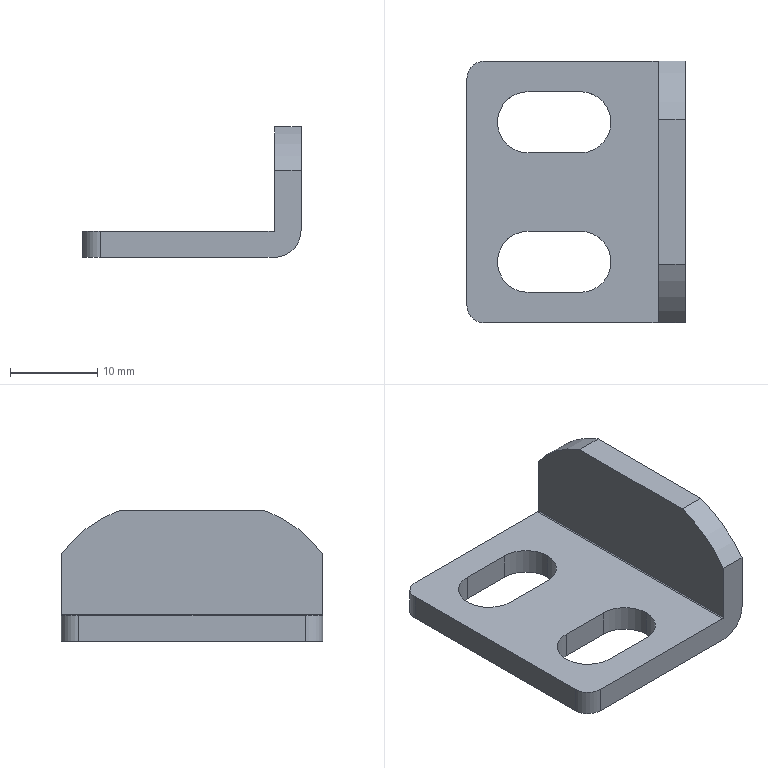Part | STEP file | X Limit Switch Bracket | 1 solid | 24 faces | box 25 x 30 x 15 mm | volume 2701 mm3 | cylinder 12 | plane 12 | commonest cylinder face diameters 7 x6 4 x2 28.772 x2 0.2 x1 6.2 x1
STEP:
#1=CARTESIAN_POINT('',(-2.594,-41.207,-3.));
#2=VERTEX_POINT('',#1);
#3=CARTESIAN_POINT('',(-6.094,-37.707,-3.));
#4=VERTEX_POINT('',#3);
#5=CARTESIAN_POINT('',(-6.094,-41.207,-3.));
#6=DIRECTION('',(0.,0.,1.));
#7=DIRECTION('',(1.,0.,0.));
#8=AXIS2_PLACEMENT_3D('',#5,#6,#7);
#9=CIRCLE('',#8,3.5);
#10=EDGE_CURVE('',#2,#4,#9,.T.);
#11=ORIENTED_EDGE('',*,*,#10,.F.);
#12=CARTESIAN_POINT('',(-2.594,-41.207,0.));
#13=VERTEX_POINT('',#12);
#14=CARTESIAN_POINT('',(-2.594,-41.207,-10.));
#15=DIRECTION('',(0.,0.,1.));
#16=VECTOR('',#15,1000.);
#17=LINE('',#14,#16);
#18=EDGE_CURVE('',#2,#13,#17,.T.);
#19=ORIENTED_EDGE('',*,*,#18,.T.);
#20=CARTESIAN_POINT('',(-6.094,-37.707,0.));
#21=VERTEX_POINT('',#20);
#22=CARTESIAN_POINT('',(-6.094,-41.207,0.));
#23=DIRECTION('',(0.,0.,-1.));
#24=DIRECTION('',(1.,0.,0.));
#25=AXIS2_PLACEMENT_3D('',#22,#23,#24);
#26=CIRCLE('',#25,3.5);
#27=EDGE_CURVE('',#21,#13,#26,.T.);
#28=ORIENTED_EDGE('',*,*,#27,.F.);
#29=CARTESIAN_POINT('',(-6.094,-37.707,-10.));
#30=DIRECTION('',(0.,0.,1.));
#31=VECTOR('',#30,1000.);
#32=LINE('',#29,#31);
#33=EDGE_CURVE('',#4,#21,#32,.T.);
#34=ORIENTED_EDGE('',*,*,#33,.F.);
#35=EDGE_LOOP('',(#11,#19,#28,#34));
#36=FACE_OUTER_BOUND('',#35,.T.);
#37=CARTESIAN_POINT('',(-6.094,-41.207,-10.));
#38=DIRECTION('',(0.,0.,1.));
#39=DIRECTION('',(1.,0.,0.));
#40=AXIS2_PLACEMENT_3D('',#37,#38,#39);
#41=CYLINDRICAL_SURFACE('',#40,3.5);
#42=ADVANCED_FACE('',(#36),#41,.F.);
#43=CARTESIAN_POINT('',(-2.594,-57.207,-3.));
#44=VERTEX_POINT('',#43);
#45=CARTESIAN_POINT('',(-6.094,-53.707,-3.));
#46=VERTEX_POINT('',#45);
#47=CARTESIAN_POINT('',(-6.094,-57.207,-3.));
#48=DIRECTION('',(0.,0.,1.));
#49=DIRECTION('',(1.,0.,0.));
#50=AXIS2_PLACEMENT_3D('',#47,#48,#49);
#51=CIRCLE('',#50,3.5);
#52=EDGE_CURVE('',#44,#46,#51,.T.);
#53=ORIENTED_EDGE('',*,*,#52,.F.);
#54=CARTESIAN_POINT('',(-2.594,-57.207,0.));
#55=VERTEX_POINT('',#54);
#56=CARTESIAN_POINT('',(-2.594,-57.207,-10.));
#57=DIRECTION('',(0.,0.,1.));
#58=VECTOR('',#57,1000.);
#59=LINE('',#56,#58);
#60=EDGE_CURVE('',#44,#55,#59,.T.);
#61=ORIENTED_EDGE('',*,*,#60,.T.);
#62=CARTESIAN_POINT('',(-6.094,-53.707,0.));
#63=VERTEX_POINT('',#62);
#64=CARTESIAN_POINT('',(-6.094,-57.207,0.));
#65=DIRECTION('',(0.,0.,-1.));
#66=DIRECTION('',(1.,0.,0.));
#67=AXIS2_PLACEMENT_3D('',#64,#65,#66);
#68=CIRCLE('',#67,3.5);
#69=EDGE_CURVE('',#63,#55,#68,.T.);
#70=ORIENTED_EDGE('',*,*,#69,.F.);
#71=CARTESIAN_POINT('',(-6.094,-53.707,-10.));
#72=DIRECTION('',(0.,0.,1.));
#73=VECTOR('',#72,1000.);
#74=LINE('',#71,#73);
#75=EDGE_CURVE('',#46,#63,#74,.T.);
#76=ORIENTED_EDGE('',*,*,#75,.F.);
#77=EDGE_LOOP('',(#53,#61,#70,#76));
#78=FACE_OUTER_BOUND('',#77,.T.);
#79=CARTESIAN_POINT('',(-6.094,-57.207,-10.));
#80=DIRECTION('',(0.,0.,1.));
#81=DIRECTION('',(1.,0.,0.));
#82=AXIS2_PLACEMENT_3D('',#79,#80,#81);
#83=CYLINDRICAL_SURFACE('',#82,3.5);
#84=ADVANCED_FACE('',(#78),#83,.F.);
#85=CARTESIAN_POINT('',(-17.094,-64.207,0.));
#86=VERTEX_POINT('',#85);
#87=CARTESIAN_POINT('',(2.806,-64.207,0.));
#88=VERTEX_POINT('',#87);
#89=CARTESIAN_POINT('',(0.,-64.207,0.));
#90=DIRECTION('',(1.,0.,0.));
#91=VECTOR('',#90,1000.);
#92=LINE('',#89,#91);
#93=EDGE_CURVE('',#86,#88,#92,.T.);
#94=ORIENTED_EDGE('',*,*,#93,.T.);
#95=CARTESIAN_POINT('',(2.806,-34.207,0.));
#96=VERTEX_POINT('',#95);
#97=CARTESIAN_POINT('',(2.806,0.,0.));
#98=DIRECTION('',(0.,1.,0.));
#99=VECTOR('',#98,1000.);
#100=LINE('',#97,#99);
#101=EDGE_CURVE('',#88,#96,#100,.T.);
#102=ORIENTED_EDGE('',*,*,#101,.T.);
#103=CARTESIAN_POINT('',(-17.094,-34.207,0.));
#104=VERTEX_POINT('',#103);
#105=CARTESIAN_POINT('',(0.,-34.207,0.));
#106=DIRECTION('',(-1.,0.,0.));
#107=VECTOR('',#106,1000.);
#108=LINE('',#105,#107);
#109=EDGE_CURVE('',#96,#104,#108,.T.);
#110=ORIENTED_EDGE('',*,*,#109,.T.);
#111=CARTESIAN_POINT('',(-19.094,-36.207,0.));
#112=VERTEX_POINT('',#111);
#113=CARTESIAN_POINT('',(-17.094,-36.207,0.));
#114=DIRECTION('',(0.,0.,1.));
#115=DIRECTION('',(1.,0.,0.));
#116=AXIS2_PLACEMENT_3D('',#113,#114,#115);
#117=CIRCLE('',#116,2.);
#118=EDGE_CURVE('',#104,#112,#117,.T.);
#119=ORIENTED_EDGE('',*,*,#118,.T.);
#120=CARTESIAN_POINT('',(-19.094,-62.207,0.));
#121=VERTEX_POINT('',#120);
#122=CARTESIAN_POINT('',(-19.094,0.,0.));
#123=DIRECTION('',(0.,-1.,0.));
#124=VECTOR('',#123,1000.);
#125=LINE('',#122,#124);
#126=EDGE_CURVE('',#112,#121,#125,.T.);
#127=ORIENTED_EDGE('',*,*,#126,.T.);
#128=CARTESIAN_POINT('',(-17.094,-62.207,0.));
#129=DIRECTION('',(0.,0.,1.));
#130=DIRECTION('',(1.,0.,0.));
#131=AXIS2_PLACEMENT_3D('',#128,#129,#130);
#132=CIRCLE('',#131,2.);
#133=EDGE_CURVE('',#121,#86,#132,.T.);
#134=ORIENTED_EDGE('',*,*,#133,.T.);
#135=EDGE_LOOP('',(#94,#102,#110,#119,#127,#134));
#136=FACE_OUTER_BOUND('',#135,.T.);
#137=ORIENTED_EDGE('',*,*,#27,.T.);
#138=CARTESIAN_POINT('',(-6.094,-44.707,0.));
#139=VERTEX_POINT('',#138);
#140=CARTESIAN_POINT('',(-6.094,-41.207,0.));
#141=DIRECTION('',(0.,0.,-1.));
#142=DIRECTION('',(1.,0.,0.));
#143=AXIS2_PLACEMENT_3D('',#140,#141,#142);
#144=CIRCLE('',#143,3.5);
#145=EDGE_CURVE('',#13,#139,#144,.T.);
#146=ORIENTED_EDGE('',*,*,#145,.T.);
#147=CARTESIAN_POINT('',(-12.094,-44.707,0.));
#148=VERTEX_POINT('',#147);
#149=CARTESIAN_POINT('',(0.,-44.707,0.));
#150=DIRECTION('',(-1.,0.,0.));
#151=VECTOR('',#150,1000.);
#152=LINE('',#149,#151);
#153=EDGE_CURVE('',#139,#148,#152,.T.);
#154=ORIENTED_EDGE('',*,*,#153,.T.);
#155=CARTESIAN_POINT('',(-12.094,-37.707,0.));
#156=VERTEX_POINT('',#155);
#157=CARTESIAN_POINT('',(-12.094,-41.207,0.));
#158=DIRECTION('',(0.,0.,-1.));
#159=DIRECTION('',(1.,0.,0.));
#160=AXIS2_PLACEMENT_3D('',#157,#158,#159);
#161=CIRCLE('',#160,3.5);
#162=EDGE_CURVE('',#148,#156,#161,.T.);
#163=ORIENTED_EDGE('',*,*,#162,.T.);
#164=CARTESIAN_POINT('',(0.,-37.707,0.));
#165=DIRECTION('',(1.,0.,0.));
#166=VECTOR('',#165,1000.);
#167=LINE('',#164,#166);
#168=EDGE_CURVE('',#156,#21,#167,.T.);
#169=ORIENTED_EDGE('',*,*,#168,.T.);
#170=EDGE_LOOP('',(#137,#146,#154,#163,#169));
#171=FACE_BOUND('',#170,.T.);
#172=ORIENTED_EDGE('',*,*,#69,.T.);
#173=CARTESIAN_POINT('',(-6.094,-60.707,0.));
#174=VERTEX_POINT('',#173);
#175=CARTESIAN_POINT('',(-6.094,-57.207,0.));
#176=DIRECTION('',(0.,0.,-1.));
#177=DIRECTION('',(1.,0.,0.));
#178=AXIS2_PLACEMENT_3D('',#175,#176,#177);
#179=CIRCLE('',#178,3.5);
#180=EDGE_CURVE('',#55,#174,#179,.T.);
#181=ORIENTED_EDGE('',*,*,#180,.T.);
#182=CARTESIAN_POINT('',(-12.094,-60.707,0.));
#183=VERTEX_POINT('',#182);
#184=CARTESIAN_POINT('',(0.,-60.707,0.));
#185=DIRECTION('',(-1.,0.,0.));
#186=VECTOR('',#185,1000.);
#187=LINE('',#184,#186);
#188=EDGE_CURVE('',#174,#183,#187,.T.);
#189=ORIENTED_EDGE('',*,*,#188,.T.);
#190=CARTESIAN_POINT('',(-12.094,-53.707,0.));
#191=VERTEX_POINT('',#190);
#192=CARTESIAN_POINT('',(-12.094,-57.207,0.));
#193=DIRECTION('',(0.,0.,-1.));
#194=DIRECTION('',(1.,0.,0.));
#195=AXIS2_PLACEMENT_3D('',#192,#193,#194);
#196=CIRCLE('',#195,3.5);
#197=EDGE_CURVE('',#183,#191,#196,.T.);
#198=ORIENTED_EDGE('',*,*,#197,.T.);
#199=CARTESIAN_POINT('',(0.,-53.707,0.));
#200=DIRECTION('',(1.,0.,0.));
#201=VECTOR('',#200,1000.);
#202=LINE('',#199,#201);
#203=EDGE_CURVE('',#191,#63,#202,.T.);
#204=ORIENTED_EDGE('',*,*,#203,.T.);
#205=EDGE_LOOP('',(#172,#181,#189,#198,#204));
#206=FACE_BOUND('',#205,.T.);
#207=CARTESIAN_POINT('',(0.,0.,0.));
#208=DIRECTION('',(0.,0.,1.));
#209=DIRECTION('',(1.,0.,0.));
#210=AXIS2_PLACEMENT_3D('',#207,#208,#209);
#211=PLANE('',#210);
#212=ADVANCED_FACE('',(#136,#171,#206),#211,.T.);
#213=CARTESIAN_POINT('',(2.906,-64.207,0.1));
#214=VERTEX_POINT('',#213);
#215=CARTESIAN_POINT('',(2.806,-64.207,0.1));
#216=DIRECTION('',(0.,1.,0.));
#217=DIRECTION('',(0.,0.,1.));
#218=AXIS2_PLACEMENT_3D('',#215,#216,#217);
#219=CIRCLE('',#218,0.1);
#220=EDGE_CURVE('',#214,#88,#219,.T.);
#221=ORIENTED_EDGE('',*,*,#220,.F.);
#222=CARTESIAN_POINT('',(2.906,-34.207,0.1));
#223=VERTEX_POINT('',#222);
#224=CARTESIAN_POINT('',(2.906,-34.207,0.1));
#225=DIRECTION('',(0.,-1.,0.));
#226=VECTOR('',#225,1000.);
#227=LINE('',#224,#226);
#228=EDGE_CURVE('',#223,#214,#227,.T.);
#229=ORIENTED_EDGE('',*,*,#228,.F.);
#230=CARTESIAN_POINT('',(2.806,-34.207,0.1));
#231=DIRECTION('',(0.,1.,0.));
#232=DIRECTION('',(0.,0.,1.));
#233=AXIS2_PLACEMENT_3D('',#230,#231,#232);
#234=CIRCLE('',#233,0.1);
#235=EDGE_CURVE('',#223,#96,#234,.T.);
#236=ORIENTED_EDGE('',*,*,#235,.T.);
#237=ORIENTED_EDGE('',*,*,#101,.F.);
#238=EDGE_LOOP('',(#221,#229,#236,#237));
#239=FACE_OUTER_BOUND('',#238,.T.);
#240=CARTESIAN_POINT('',(2.806,-34.207,0.1));
#241=DIRECTION('',(0.,1.,0.));
#242=DIRECTION('',(0.,0.,1.));
#243=AXIS2_PLACEMENT_3D('',#240,#241,#242);
#244=CYLINDRICAL_SURFACE('',#243,0.1);
#245=ADVANCED_FACE('',(#239),#244,.F.);
#246=CARTESIAN_POINT('',(-17.094,-64.207,-3.));
#247=VERTEX_POINT('',#246);
#248=CARTESIAN_POINT('',(2.806,-64.207,-3.));
#249=VERTEX_POINT('',#248);
#250=CARTESIAN_POINT('',(-19.094,-64.207,-3.));
#251=DIRECTION('',(1.,0.,0.));
#252=VECTOR('',#251,1000.);
#253=LINE('',#250,#252);
#254=EDGE_CURVE('',#247,#249,#253,.T.);
#255=ORIENTED_EDGE('',*,*,#254,.T.);
#256=CARTESIAN_POINT('',(5.906,-64.207,0.1));
#257=VERTEX_POINT('',#256);
#258=CARTESIAN_POINT('',(2.806,-64.207,0.1));
#259=DIRECTION('',(0.,-1.,0.));
#260=DIRECTION('',(0.,0.,1.));
#261=AXIS2_PLACEMENT_3D('',#258,#259,#260);
#262=CIRCLE('',#261,3.1);
#263=EDGE_CURVE('',#249,#257,#262,.T.);
#264=ORIENTED_EDGE('',*,*,#263,.T.);
#265=CARTESIAN_POINT('',(5.906,-64.207,7.));
#266=VERTEX_POINT('',#265);
#267=CARTESIAN_POINT('',(5.906,-64.207,0.));
#268=DIRECTION('',(0.,0.,-1.));
#269=VECTOR('',#268,1000.);
#270=LINE('',#267,#269);
#271=EDGE_CURVE('',#266,#257,#270,.T.);
#272=ORIENTED_EDGE('',*,*,#271,.F.);
#273=CARTESIAN_POINT('',(2.906,-64.207,7.));
#274=VERTEX_POINT('',#273);
#275=CARTESIAN_POINT('',(5.906,-64.207,7.));
#276=DIRECTION('',(1.,0.,0.));
#277=VECTOR('',#276,1000.);
#278=LINE('',#275,#277);
#279=EDGE_CURVE('',#274,#266,#278,.T.);
#280=ORIENTED_EDGE('',*,*,#279,.F.);
#281=CARTESIAN_POINT('',(2.906,-64.207,0.));
#282=DIRECTION('',(0.,0.,1.));
#283=VECTOR('',#282,1000.);
#284=LINE('',#281,#283);
#285=EDGE_CURVE('',#214,#274,#284,.T.);
#286=ORIENTED_EDGE('',*,*,#285,.F.);
#287=ORIENTED_EDGE('',*,*,#220,.T.);
#288=ORIENTED_EDGE('',*,*,#93,.F.);
#289=CARTESIAN_POINT('',(-17.094,-64.207,-3.));
#290=DIRECTION('',(0.,0.,-1.));
#291=VECTOR('',#290,1000.);
#292=LINE('',#289,#291);
#293=EDGE_CURVE('',#86,#247,#292,.T.);
#294=ORIENTED_EDGE('',*,*,#293,.T.);
#295=EDGE_LOOP('',(#255,#264,#272,#280,#286,#287,#288,#294));
#296=FACE_OUTER_BOUND('',#295,.T.);
#297=CARTESIAN_POINT('',(-19.094,-64.207,-3.));
#298=DIRECTION('',(0.,-1.,0.));
#299=DIRECTION('',(0.,0.,-1.));
#300=AXIS2_PLACEMENT_3D('',#297,#298,#299);
#301=PLANE('',#300);
#302=ADVANCED_FACE('',(#296),#301,.T.);
#303=ORIENTED_EDGE('',*,*,#133,.F.);
#304=CARTESIAN_POINT('',(-19.094,-62.207,-3.));
#305=VERTEX_POINT('',#304);
#306=CARTESIAN_POINT('',(-19.094,-62.207,-3.));
#307=DIRECTION('',(0.,0.,-1.));
#308=VECTOR('',#307,1000.);
#309=LINE('',#306,#308);
#310=EDGE_CURVE('',#121,#305,#309,.T.);
#311=ORIENTED_EDGE('',*,*,#310,.T.);
#312=CARTESIAN_POINT('',(-17.094,-62.207,-3.));
#313=DIRECTION('',(0.,0.,1.));
#314=DIRECTION('',(1.,0.,0.));
#315=AXIS2_PLACEMENT_3D('',#312,#313,#314);
#316=CIRCLE('',#315,2.);
#317=EDGE_CURVE('',#305,#247,#316,.T.);
#318=ORIENTED_EDGE('',*,*,#317,.T.);
#319=ORIENTED_EDGE('',*,*,#293,.F.);
#320=EDGE_LOOP('',(#303,#311,#318,#319));
#321=FACE_OUTER_BOUND('',#320,.T.);
#322=CARTESIAN_POINT('',(-17.094,-62.207,-3.));
#323=DIRECTION('',(0.,0.,1.));
#324=DIRECTION('',(1.,0.,0.));
#325=AXIS2_PLACEMENT_3D('',#322,#323,#324);
#326=CYLINDRICAL_SURFACE('',#325,2.);
#327=ADVANCED_FACE('',(#321),#326,.T.);
#328=CARTESIAN_POINT('',(-19.094,-36.207,-3.));
#329=VERTEX_POINT('',#328);
#330=CARTESIAN_POINT('',(-19.094,-34.207,-3.));
#331=DIRECTION('',(0.,-1.,0.));
#332=VECTOR('',#331,1000.);
#333=LINE('',#330,#332);
#334=EDGE_CURVE('',#329,#305,#333,.T.);
#335=ORIENTED_EDGE('',*,*,#334,.T.);
#336=ORIENTED_EDGE('',*,*,#310,.F.);
#337=ORIENTED_EDGE('',*,*,#126,.F.);
#338=CARTESIAN_POINT('',(-19.094,-36.207,-3.));
#339=DIRECTION('',(0.,0.,-1.));
#340=VECTOR('',#339,1000.);
#341=LINE('',#338,#340);
#342=EDGE_CURVE('',#112,#329,#341,.T.);
#343=ORIENTED_EDGE('',*,*,#342,.T.);
#344=EDGE_LOOP('',(#335,#336,#337,#343));
#345=FACE_OUTER_BOUND('',#344,.T.);
#346=CARTESIAN_POINT('',(-19.094,-34.207,-3.));
#347=DIRECTION('',(-1.,0.,0.));
#348=DIRECTION('',(0.,-1.,0.));
#349=AXIS2_PLACEMENT_3D('',#346,#347,#348);
#350=PLANE('',#349);
#351=ADVANCED_FACE('',(#345),#350,.T.);
#352=ORIENTED_EDGE('',*,*,#118,.F.);
#353=CARTESIAN_POINT('',(-17.094,-34.207,-3.));
#354=VERTEX_POINT('',#353);
#355=CARTESIAN_POINT('',(-17.094,-34.207,-3.));
#356=DIRECTION('',(0.,0.,-1.));
#357=VECTOR('',#356,1000.);
#358=LINE('',#355,#357);
#359=EDGE_CURVE('',#104,#354,#358,.T.);
#360=ORIENTED_EDGE('',*,*,#359,.T.);
#361=CARTESIAN_POINT('',(-17.094,-36.207,-3.));
#362=DIRECTION('',(0.,0.,1.));
#363=DIRECTION('',(1.,0.,0.));
#364=AXIS2_PLACEMENT_3D('',#361,#362,#363);
#365=CIRCLE('',#364,2.);
#366=EDGE_CURVE('',#354,#329,#365,.T.);
#367=ORIENTED_EDGE('',*,*,#366,.T.);
#368=ORIENTED_EDGE('',*,*,#342,.F.);
#369=EDGE_LOOP('',(#352,#360,#367,#368));
#370=FACE_OUTER_BOUND('',#369,.T.);
#371=CARTESIAN_POINT('',(-17.094,-36.207,-3.));
#372=DIRECTION('',(0.,0.,1.));
#373=DIRECTION('',(1.,0.,0.));
#374=AXIS2_PLACEMENT_3D('',#371,#372,#373);
#375=CYLINDRICAL_SURFACE('',#374,2.);
#376=ADVANCED_FACE('',(#370),#375,.T.);
#377=ORIENTED_EDGE('',*,*,#109,.F.);
#378=ORIENTED_EDGE('',*,*,#235,.F.);
#379=CARTESIAN_POINT('',(2.906,-34.207,7.));
#380=VERTEX_POINT('',#379);
#381=CARTESIAN_POINT('',(2.906,-34.207,0.));
#382=DIRECTION('',(0.,0.,-1.));
#383=VECTOR('',#382,1000.);
#384=LINE('',#381,#383);
#385=EDGE_CURVE('',#380,#223,#384,.T.);
#386=ORIENTED_EDGE('',*,*,#385,.F.);
#387=CARTESIAN_POINT('',(5.906,-34.207,7.));
#388=VERTEX_POINT('',#387);
#389=CARTESIAN_POINT('',(5.906,-34.207,7.));
#390=DIRECTION('',(-1.,0.,0.));
#391=VECTOR('',#390,1000.);
#392=LINE('',#389,#391);
#393=EDGE_CURVE('',#388,#380,#392,.T.);
#394=ORIENTED_EDGE('',*,*,#393,.F.);
#395=CARTESIAN_POINT('',(5.906,-34.207,0.1));
#396=VERTEX_POINT('',#395);
#397=CARTESIAN_POINT('',(5.906,-34.207,12.));
#398=DIRECTION('',(0.,0.,1.));
#399=VECTOR('',#398,1000.);
#400=LINE('',#397,#399);
#401=EDGE_CURVE('',#396,#388,#400,.T.);
#402=ORIENTED_EDGE('',*,*,#401,.F.);
#403=CARTESIAN_POINT('',(2.806,-34.207,-3.));
#404=VERTEX_POINT('',#403);
#405=CARTESIAN_POINT('',(2.806,-34.207,0.1));
#406=DIRECTION('',(0.,-1.,0.));
#407=DIRECTION('',(0.,0.,1.));
#408=AXIS2_PLACEMENT_3D('',#405,#406,#407);
#409=CIRCLE('',#408,3.1);
#410=EDGE_CURVE('',#404,#396,#409,.T.);
#411=ORIENTED_EDGE('',*,*,#410,.F.);
#412=CARTESIAN_POINT('',(-19.094,-34.207,-3.));
#413=DIRECTION('',(-1.,0.,0.));
#414=VECTOR('',#413,1000.);
#415=LINE('',#412,#414);
#416=EDGE_CURVE('',#404,#354,#415,.T.);
#417=ORIENTED_EDGE('',*,*,#416,.T.);
#418=ORIENTED_EDGE('',*,*,#359,.F.);
#419=EDGE_LOOP('',(#377,#378,#386,#394,#402,#411,#417,#418));
#420=FACE_OUTER_BOUND('',#419,.T.);
#421=CARTESIAN_POINT('',(-19.094,-34.207,-3.));
#422=DIRECTION('',(0.,1.,0.));
#423=DIRECTION('',(0.,0.,1.));
#424=AXIS2_PLACEMENT_3D('',#421,#422,#423);
#425=PLANE('',#424);
#426=ADVANCED_FACE('',(#420),#425,.T.);
#427=ORIENTED_EDGE('',*,*,#153,.F.);
#428=CARTESIAN_POINT('',(-6.094,-44.707,-3.));
#429=VERTEX_POINT('',#428);
#430=CARTESIAN_POINT('',(-6.094,-44.707,-10.));
#431=DIRECTION('',(0.,0.,1.));
#432=VECTOR('',#431,1000.);
#433=LINE('',#430,#432);
#434=EDGE_CURVE('',#429,#139,#433,.T.);
#435=ORIENTED_EDGE('',*,*,#434,.F.);
#436=CARTESIAN_POINT('',(-12.094,-44.707,-3.));
#437=VERTEX_POINT('',#436);
#438=CARTESIAN_POINT('',(-12.094,-44.707,-3.));
#439=DIRECTION('',(1.,0.,0.));
#440=VECTOR('',#439,1000.);
#441=LINE('',#438,#440);
#442=EDGE_CURVE('',#437,#429,#441,.T.);
#443=ORIENTED_EDGE('',*,*,#442,.F.);
#444=CARTESIAN_POINT('',(-12.094,-44.707,-10.));
#445=DIRECTION('',(0.,0.,-1.));
#446=VECTOR('',#445,1000.);
#447=LINE('',#444,#446);
#448=EDGE_CURVE('',#148,#437,#447,.T.);
#449=ORIENTED_EDGE('',*,*,#448,.F.);
#450=EDGE_LOOP('',(#427,#435,#443,#449));
#451=FACE_OUTER_BOUND('',#450,.T.);
#452=CARTESIAN_POINT('',(-12.094,-44.707,-10.));
#453=DIRECTION('',(0.,-1.,0.));
#454=DIRECTION('',(0.,0.,-1.));
#455=AXIS2_PLACEMENT_3D('',#452,#453,#454);
#456=PLANE('',#455);
#457=ADVANCED_FACE('',(#451),#456,.F.);
#458=ORIENTED_EDGE('',*,*,#18,.F.);
#459=CARTESIAN_POINT('',(-6.094,-41.207,-3.));
#460=DIRECTION('',(0.,0.,1.));
#461=DIRECTION('',(1.,0.,0.));
#462=AXIS2_PLACEMENT_3D('',#459,#460,#461);
#463=CIRCLE('',#462,3.5);
#464=EDGE_CURVE('',#429,#2,#463,.T.);
#465=ORIENTED_EDGE('',*,*,#464,.F.);
#466=ORIENTED_EDGE('',*,*,#434,.T.);
#467=ORIENTED_EDGE('',*,*,#145,.F.);
#468=EDGE_LOOP('',(#458,#465,#466,#467));
#469=FACE_OUTER_BOUND('',#468,.T.);
#470=CARTESIAN_POINT('',(-6.094,-41.207,-10.));
#471=DIRECTION('',(0.,0.,1.));
#472=DIRECTION('',(1.,0.,0.));
#473=AXIS2_PLACEMENT_3D('',#470,#471,#472);
#474=CYLINDRICAL_SURFACE('',#473,3.5);
#475=ADVANCED_FACE('',(#469),#474,.F.);
#476=ORIENTED_EDGE('',*,*,#168,.F.);
#477=CARTESIAN_POINT('',(-12.094,-37.707,-3.));
#478=VERTEX_POINT('',#477);
#479=CARTESIAN_POINT('',(-12.094,-37.707,-10.));
#480=DIRECTION('',(0.,0.,1.));
#481=VECTOR('',#480,1000.);
#482=LINE('',#479,#481);
#483=EDGE_CURVE('',#478,#156,#482,.T.);
#484=ORIENTED_EDGE('',*,*,#483,.F.);
#485=CARTESIAN_POINT('',(-12.094,-37.707,-3.));
#486=DIRECTION('',(-1.,0.,0.));
#487=VECTOR('',#486,1000.);
#488=LINE('',#485,#487);
#489=EDGE_CURVE('',#4,#478,#488,.T.);
#490=ORIENTED_EDGE('',*,*,#489,.F.);
#491=ORIENTED_EDGE('',*,*,#33,.T.);
#492=EDGE_LOOP('',(#476,#484,#490,#491));
#493=FACE_OUTER_BOUND('',#492,.T.);
#494=CARTESIAN_POINT('',(-12.094,-37.707,-10.));
#495=DIRECTION('',(0.,1.,0.));
#496=DIRECTION('',(0.,0.,1.));
#497=AXIS2_PLACEMENT_3D('',#494,#495,#496);
#498=PLANE('',#497);
#499=ADVANCED_FACE('',(#493),#498,.F.);
#500=ORIENTED_EDGE('',*,*,#162,.F.);
#501=ORIENTED_EDGE('',*,*,#448,.T.);
#502=CARTESIAN_POINT('',(-12.094,-41.207,-3.));
#503=DIRECTION('',(0.,0.,1.));
#504=DIRECTION('',(1.,0.,0.));
#505=AXIS2_PLACEMENT_3D('',#502,#503,#504);
#506=CIRCLE('',#505,3.5);
#507=EDGE_CURVE('',#478,#437,#506,.T.);
#508=ORIENTED_EDGE('',*,*,#507,.F.);
#509=ORIENTED_EDGE('',*,*,#483,.T.);
#510=EDGE_LOOP('',(#500,#501,#508,#509));
#511=FACE_OUTER_BOUND('',#510,.T.);
#512=CARTESIAN_POINT('',(-12.094,-41.207,-10.));
#513=DIRECTION('',(0.,0.,1.));
#514=DIRECTION('',(1.,0.,0.));
#515=AXIS2_PLACEMENT_3D('',#512,#513,#514);
#516=CYLINDRICAL_SURFACE('',#515,3.5);
#517=ADVANCED_FACE('',(#511),#516,.F.);
#518=ORIENTED_EDGE('',*,*,#188,.F.);
#519=CARTESIAN_POINT('',(-6.094,-60.707,-3.));
#520=VERTEX_POINT('',#519);
#521=CARTESIAN_POINT('',(-6.094,-60.707,-10.));
#522=DIRECTION('',(0.,0.,1.));
#523=VECTOR('',#522,1000.);
#524=LINE('',#521,#523);
#525=EDGE_CURVE('',#520,#174,#524,.T.);
#526=ORIENTED_EDGE('',*,*,#525,.F.);
#527=CARTESIAN_POINT('',(-12.094,-60.707,-3.));
#528=VERTEX_POINT('',#527);
#529=CARTESIAN_POINT('',(-12.094,-60.707,-3.));
#530=DIRECTION('',(1.,0.,0.));
#531=VECTOR('',#530,1000.);
#532=LINE('',#529,#531);
#533=EDGE_CURVE('',#528,#520,#532,.T.);
#534=ORIENTED_EDGE('',*,*,#533,.F.);
#535=CARTESIAN_POINT('',(-12.094,-60.707,-10.));
#536=DIRECTION('',(0.,0.,-1.));
#537=VECTOR('',#536,1000.);
#538=LINE('',#535,#537);
#539=EDGE_CURVE('',#183,#528,#538,.T.);
#540=ORIENTED_EDGE('',*,*,#539,.F.);
#541=EDGE_LOOP('',(#518,#526,#534,#540));
#542=FACE_OUTER_BOUND('',#541,.T.);
#543=CARTESIAN_POINT('',(-12.094,-60.707,-10.));
#544=DIRECTION('',(0.,-1.,0.));
#545=DIRECTION('',(0.,0.,-1.));
#546=AXIS2_PLACEMENT_3D('',#543,#544,#545);
#547=PLANE('',#546);
#548=ADVANCED_FACE('',(#542),#547,.F.);
#549=ORIENTED_EDGE('',*,*,#60,.F.);
#550=CARTESIAN_POINT('',(-6.094,-57.207,-3.));
#551=DIRECTION('',(0.,0.,1.));
#552=DIRECTION('',(1.,0.,0.));
#553=AXIS2_PLACEMENT_3D('',#550,#551,#552);
#554=CIRCLE('',#553,3.5);
#555=EDGE_CURVE('',#520,#44,#554,.T.);
#556=ORIENTED_EDGE('',*,*,#555,.F.);
#557=ORIENTED_EDGE('',*,*,#525,.T.);
#558=ORIENTED_EDGE('',*,*,#180,.F.);
#559=EDGE_LOOP('',(#549,#556,#557,#558));
#560=FACE_OUTER_BOUND('',#559,.T.);
#561=CARTESIAN_POINT('',(-6.094,-57.207,-10.));
#562=DIRECTION('',(0.,0.,1.));
#563=DIRECTION('',(1.,0.,0.));
#564=AXIS2_PLACEMENT_3D('',#561,#562,#563);
#565=CYLINDRICAL_SURFACE('',#564,3.5);
#566=ADVANCED_FACE('',(#560),#565,.F.);
#567=ORIENTED_EDGE('',*,*,#203,.F.);
#568=CARTESIAN_POINT('',(-12.094,-53.707,-3.));
#569=VERTEX_POINT('',#568);
#570=CARTESIAN_POINT('',(-12.094,-53.707,-10.));
#571=DIRECTION('',(0.,0.,1.));
#572=VECTOR('',#571,1000.);
#573=LINE('',#570,#572);
#574=EDGE_CURVE('',#569,#191,#573,.T.);
#575=ORIENTED_EDGE('',*,*,#574,.F.);
#576=CARTESIAN_POINT('',(-12.094,-53.707,-3.));
#577=DIRECTION('',(-1.,0.,0.));
#578=VECTOR('',#577,1000.);
#579=LINE('',#576,#578);
#580=EDGE_CURVE('',#46,#569,#579,.T.);
#581=ORIENTED_EDGE('',*,*,#580,.F.);
#582=ORIENTED_EDGE('',*,*,#75,.T.);
#583=EDGE_LOOP('',(#567,#575,#581,#582));
#584=FACE_OUTER_BOUND('',#583,.T.);
#585=CARTESIAN_POINT('',(-12.094,-53.707,-10.));
#586=DIRECTION('',(0.,1.,0.));
#587=DIRECTION('',(0.,0.,1.));
#588=AXIS2_PLACEMENT_3D('',#585,#586,#587);
#589=PLANE('',#588);
#590=ADVANCED_FACE('',(#584),#589,.F.);
#591=ORIENTED_EDGE('',*,*,#197,.F.);
#592=ORIENTED_EDGE('',*,*,#539,.T.);
#593=CARTESIAN_POINT('',(-12.094,-57.207,-3.));
#594=DIRECTION('',(0.,0.,1.));
#595=DIRECTION('',(1.,0.,0.));
#596=AXIS2_PLACEMENT_3D('',#593,#594,#595);
#597=CIRCLE('',#596,3.5);
#598=EDGE_CURVE('',#569,#528,#597,.T.);
#599=ORIENTED_EDGE('',*,*,#598,.F.);
#600=ORIENTED_EDGE('',*,*,#574,.T.);
#601=EDGE_LOOP('',(#591,#592,#599,#600));
#602=FACE_OUTER_BOUND('',#601,.T.);
#603=CARTESIAN_POINT('',(-12.094,-57.207,-10.));
#604=DIRECTION('',(0.,0.,1.));
#605=DIRECTION('',(1.,0.,0.));
#606=AXIS2_PLACEMENT_3D('',#603,#604,#605);
#607=CYLINDRICAL_SURFACE('',#606,3.5);
#608=ADVANCED_FACE('',(#602),#607,.F.);
#609=ORIENTED_EDGE('',*,*,#285,.T.);
#610=CARTESIAN_POINT('',(2.906,-57.525,12.));
#611=VERTEX_POINT('',#610);
#612=CARTESIAN_POINT('',(2.906,-52.617,-1.523));
#613=DIRECTION('',(-1.,0.,0.));
#614=DIRECTION('',(0.,0.,1.));
#615=AXIS2_PLACEMENT_3D('',#612,#613,#614);
#616=CIRCLE('',#615,14.386);
#617=EDGE_CURVE('',#274,#611,#616,.T.);
#618=ORIENTED_EDGE('',*,*,#617,.T.);
#619=CARTESIAN_POINT('',(2.906,-40.888,12.));
#620=VERTEX_POINT('',#619);
#621=CARTESIAN_POINT('',(2.906,0.,12.));
#622=DIRECTION('',(0.,1.,0.));
#623=VECTOR('',#622,1000.);
#624=LINE('',#621,#623);
#625=EDGE_CURVE('',#611,#620,#624,.T.);
#626=ORIENTED_EDGE('',*,*,#625,.T.);
#627=CARTESIAN_POINT('',(2.906,-45.796,-1.523));
#628=DIRECTION('',(-1.,0.,0.));
#629=DIRECTION('',(0.,0.,1.));
#630=AXIS2_PLACEMENT_3D('',#627,#628,#629);
#631=CIRCLE('',#630,14.386);
#632=EDGE_CURVE('',#620,#380,#631,.T.);
#633=ORIENTED_EDGE('',*,*,#632,.T.);
#634=ORIENTED_EDGE('',*,*,#385,.T.);
#635=ORIENTED_EDGE('',*,*,#228,.T.);
#636=EDGE_LOOP('',(#609,#618,#626,#633,#634,#635));
#637=FACE_OUTER_BOUND('',#636,.T.);
#638=CARTESIAN_POINT('',(2.906,0.,0.));
#639=DIRECTION('',(-1.,0.,0.));
#640=DIRECTION('',(0.,0.,1.));
#641=AXIS2_PLACEMENT_3D('',#638,#639,#640);
#642=PLANE('',#641);
#643=ADVANCED_FACE('',(#637),#642,.T.);
#644=ORIENTED_EDGE('',*,*,#366,.F.);
#645=ORIENTED_EDGE('',*,*,#416,.F.);
#646=CARTESIAN_POINT('',(2.806,0.,-3.));
#647=DIRECTION('',(0.,1.,0.));
#648=VECTOR('',#647,1000.);
#649=LINE('',#646,#648);
#650=EDGE_CURVE('',#249,#404,#649,.T.);
#651=ORIENTED_EDGE('',*,*,#650,.F.);
#652=ORIENTED_EDGE('',*,*,#254,.F.);
#653=ORIENTED_EDGE('',*,*,#317,.F.);
#654=ORIENTED_EDGE('',*,*,#334,.F.);
#655=EDGE_LOOP('',(#644,#645,#651,#652,#653,#654));
#656=FACE_OUTER_BOUND('',#655,.T.);
#657=ORIENTED_EDGE('',*,*,#507,.T.);
#658=ORIENTED_EDGE('',*,*,#442,.T.);
#659=ORIENTED_EDGE('',*,*,#464,.T.);
#660=ORIENTED_EDGE('',*,*,#10,.T.);
#661=ORIENTED_EDGE('',*,*,#489,.T.);
#662=EDGE_LOOP('',(#657,#658,#659,#660,#661));
#663=FACE_BOUND('',#662,.T.);
#664=ORIENTED_EDGE('',*,*,#598,.T.);
#665=ORIENTED_EDGE('',*,*,#533,.T.);
#666=ORIENTED_EDGE('',*,*,#555,.T.);
#667=ORIENTED_EDGE('',*,*,#52,.T.);
#668=ORIENTED_EDGE('',*,*,#580,.T.);
#669=EDGE_LOOP('',(#664,#665,#666,#667,#668));
#670=FACE_BOUND('',#669,.T.);
#671=CARTESIAN_POINT('',(0.,0.,-3.));
#672=DIRECTION('',(0.,0.,1.));
#673=DIRECTION('',(1.,0.,0.));
#674=AXIS2_PLACEMENT_3D('',#671,#672,#673);
#675=PLANE('',#674);
#676=ADVANCED_FACE('',(#656,#663,#670),#675,.F.);
#677=CARTESIAN_POINT('',(5.906,-57.525,12.));
#678=VERTEX_POINT('',#677);
#679=CARTESIAN_POINT('',(5.906,-57.525,12.));
#680=DIRECTION('',(-1.,0.,0.));
#681=VECTOR('',#680,1000.);
#682=LINE('',#679,#681);
#683=EDGE_CURVE('',#678,#611,#682,.T.);
#684=ORIENTED_EDGE('',*,*,#683,.T.);
#685=ORIENTED_EDGE('',*,*,#617,.F.);
#686=ORIENTED_EDGE('',*,*,#279,.T.);
#687=CARTESIAN_POINT('',(5.906,-52.617,-1.523));
#688=DIRECTION('',(-1.,0.,0.));
#689=DIRECTION('',(0.,0.,1.));
#690=AXIS2_PLACEMENT_3D('',#687,#688,#689);
#691=CIRCLE('',#690,14.386);
#692=EDGE_CURVE('',#266,#678,#691,.T.);
#693=ORIENTED_EDGE('',*,*,#692,.T.);
#694=EDGE_LOOP('',(#684,#685,#686,#693));
#695=FACE_OUTER_BOUND('',#694,.T.);
#696=CARTESIAN_POINT('',(5.906,-52.617,-1.523));
#697=DIRECTION('',(-1.,0.,0.));
#698=DIRECTION('',(0.,0.,1.));
#699=AXIS2_PLACEMENT_3D('',#696,#697,#698);
#700=CYLINDRICAL_SURFACE('',#699,14.386);
#701=ADVANCED_FACE('',(#695),#700,.T.);
#702=ORIENTED_EDGE('',*,*,#393,.T.);
#703=ORIENTED_EDGE('',*,*,#632,.F.);
#704=CARTESIAN_POINT('',(5.906,-40.888,12.));
#705=VERTEX_POINT('',#704);
#706=CARTESIAN_POINT('',(5.906,-40.888,12.));
#707=DIRECTION('',(1.,0.,0.));
#708=VECTOR('',#707,1000.);
#709=LINE('',#706,#708);
#710=EDGE_CURVE('',#620,#705,#709,.T.);
#711=ORIENTED_EDGE('',*,*,#710,.T.);
#712=CARTESIAN_POINT('',(5.906,-45.796,-1.523));
#713=DIRECTION('',(-1.,0.,0.));
#714=DIRECTION('',(0.,0.,1.));
#715=AXIS2_PLACEMENT_3D('',#712,#713,#714);
#716=CIRCLE('',#715,14.386);
#717=EDGE_CURVE('',#705,#388,#716,.T.);
#718=ORIENTED_EDGE('',*,*,#717,.T.);
#719=EDGE_LOOP('',(#702,#703,#711,#718));
#720=FACE_OUTER_BOUND('',#719,.T.);
#721=CARTESIAN_POINT('',(5.906,-45.796,-1.523));
#722=DIRECTION('',(-1.,0.,0.));
#723=DIRECTION('',(0.,0.,1.));
#724=AXIS2_PLACEMENT_3D('',#721,#722,#723);
#725=CYLINDRICAL_SURFACE('',#724,14.386);
#726=ADVANCED_FACE('',(#720),#725,.T.);
#727=ORIENTED_EDGE('',*,*,#625,.F.);
#728=ORIENTED_EDGE('',*,*,#683,.F.);
#729=CARTESIAN_POINT('',(5.906,-64.207,12.));
#730=DIRECTION('',(0.,-1.,0.));
#731=VECTOR('',#730,1000.);
#732=LINE('',#729,#731);
#733=EDGE_CURVE('',#705,#678,#732,.T.);
#734=ORIENTED_EDGE('',*,*,#733,.F.);
#735=ORIENTED_EDGE('',*,*,#710,.F.);
#736=EDGE_LOOP('',(#727,#728,#734,#735));
#737=FACE_OUTER_BOUND('',#736,.T.);
#738=CARTESIAN_POINT('',(5.906,-64.207,12.));
#739=DIRECTION('',(0.,0.,-1.));
#740=DIRECTION('',(-1.,0.,0.));
#741=AXIS2_PLACEMENT_3D('',#738,#739,#740);
#742=PLANE('',#741);
#743=ADVANCED_FACE('',(#737),#742,.F.);
#744=CARTESIAN_POINT('',(5.906,-34.207,0.1));
#745=DIRECTION('',(0.,-1.,0.));
#746=VECTOR('',#745,1000.);
#747=LINE('',#744,#746);
#748=EDGE_CURVE('',#396,#257,#747,.T.);
#749=ORIENTED_EDGE('',*,*,#748,.T.);
#750=ORIENTED_EDGE('',*,*,#263,.F.);
#751=ORIENTED_EDGE('',*,*,#650,.T.);
#752=ORIENTED_EDGE('',*,*,#410,.T.);
#753=EDGE_LOOP('',(#749,#750,#751,#752));
#754=FACE_OUTER_BOUND('',#753,.T.);
#755=CARTESIAN_POINT('',(2.806,-34.207,0.1));
#756=DIRECTION('',(0.,1.,0.));
#757=DIRECTION('',(0.,0.,1.));
#758=AXIS2_PLACEMENT_3D('',#755,#756,#757);
#759=CYLINDRICAL_SURFACE('',#758,3.1);
#760=ADVANCED_FACE('',(#754),#759,.T.);
#761=ORIENTED_EDGE('',*,*,#733,.T.);
#762=ORIENTED_EDGE('',*,*,#692,.F.);
#763=ORIENTED_EDGE('',*,*,#271,.T.);
#764=ORIENTED_EDGE('',*,*,#748,.F.);
#765=ORIENTED_EDGE('',*,*,#401,.T.);
#766=ORIENTED_EDGE('',*,*,#717,.F.);
#767=EDGE_LOOP('',(#761,#762,#763,#764,#765,#766));
#768=FACE_OUTER_BOUND('',#767,.T.);
#769=CARTESIAN_POINT('',(5.906,0.,0.));
#770=DIRECTION('',(-1.,0.,0.));
#771=DIRECTION('',(0.,0.,1.));
#772=AXIS2_PLACEMENT_3D('',#769,#770,#771);
#773=PLANE('',#772);
#774=ADVANCED_FACE('',(#768),#773,.F.);
#775=CLOSED_SHELL('',(#42,#84,#212,#245,#302,#327,#351,#376,#426,#457,#475,#499,#517,#548,#566,#590,#608,#643,#676,#701,#726,#743,#760,#774));
#776=MANIFOLD_SOLID_BREP('',#775);
#777=CARTESIAN_POINT('',(0.,0.,0.));
#778=DIRECTION('',(0.,0.,1.));
#779=DIRECTION('',(1.,0.,0.));
#780=AXIS2_PLACEMENT_3D('',#777,#778,#779);
#781=(LENGTH_UNIT()NAMED_UNIT(*)SI_UNIT(.MILLI.,.METRE.));
#782=UNCERTAINTY_MEASURE_WITH_UNIT(LENGTH_MEASURE(0.00001),#781,'','');
#783=(NAMED_UNIT(*)PLANE_ANGLE_UNIT()SI_UNIT($,.RADIAN.));
#784=(NAMED_UNIT(*)SI_UNIT($,.STERADIAN.)SOLID_ANGLE_UNIT());
#785=(GEOMETRIC_REPRESENTATION_CONTEXT(3)GLOBAL_UNCERTAINTY_ASSIGNED_CONTEXT((#782))GLOBAL_UNIT_ASSIGNED_CONTEXT((#781,#783,#784))REPRESENTATION_CONTEXT('',''));
#786=ADVANCED_BREP_SHAPE_REPRESENTATION('',(#776,#780),#785);